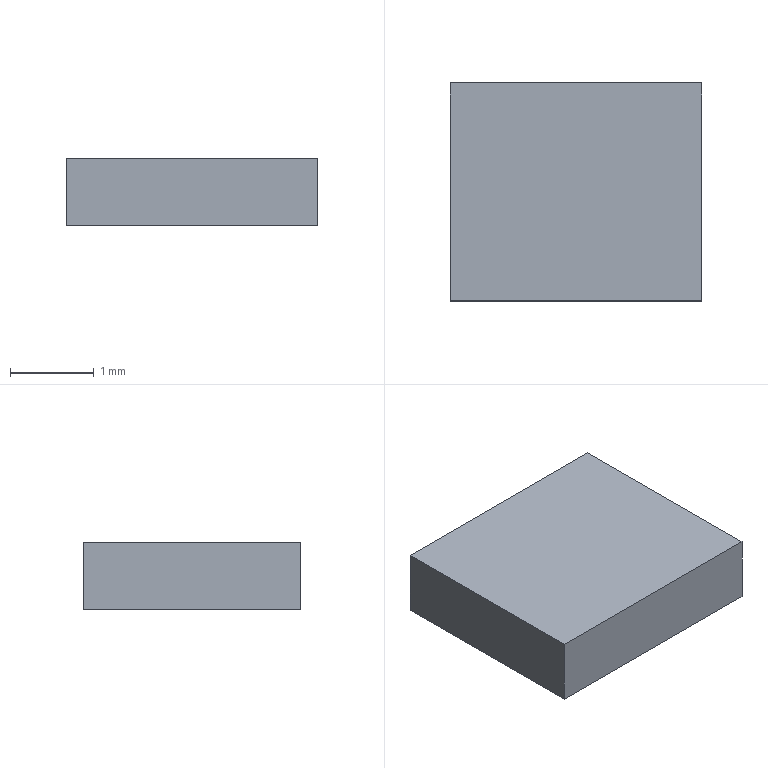Part | Creo | 1 solid | 6 faces | box 3 x 2.6 x 0.8 mm | volume 6.24 mm3 | plane 6
STEP:
#1=CARTESIAN_POINT('',(0.,0.,0.));
#2=DIRECTION('',(0.,0.,1.));
#3=DIRECTION('',(1.,0.,0.));
#4=AXIS2_PLACEMENT_3D('',#1,#2,#3);
#5=CARTESIAN_POINT('',(-1.5,1.3,0.));
#6=VERTEX_POINT('',#5);
#7=CARTESIAN_POINT('',(-1.5,-1.3,0.));
#8=VERTEX_POINT('',#7);
#9=CARTESIAN_POINT('',(-1.5,1.3,0.));
#10=DIRECTION('',(0.,-1.,0.));
#11=VECTOR('',#10,2.6);
#12=LINE('',#9,#11);
#13=EDGE_CURVE('',#6,#8,#12,.T.);
#14=ORIENTED_EDGE('',*,*,#13,.T.);
#15=CARTESIAN_POINT('',(1.5,-1.3,0.));
#16=VERTEX_POINT('',#15);
#17=CARTESIAN_POINT('',(-1.5,-1.3,0.));
#18=DIRECTION('',(1.,0.,0.));
#19=VECTOR('',#18,3.);
#20=LINE('',#17,#19);
#21=EDGE_CURVE('',#8,#16,#20,.T.);
#22=ORIENTED_EDGE('',*,*,#21,.T.);
#23=CARTESIAN_POINT('',(1.5,1.3,0.));
#24=VERTEX_POINT('',#23);
#25=CARTESIAN_POINT('',(1.5,-1.3,0.));
#26=DIRECTION('',(0.,1.,0.));
#27=VECTOR('',#26,2.6);
#28=LINE('',#25,#27);
#29=EDGE_CURVE('',#16,#24,#28,.T.);
#30=ORIENTED_EDGE('',*,*,#29,.T.);
#31=CARTESIAN_POINT('',(1.5,1.3,0.));
#32=DIRECTION('',(-1.,0.,0.));
#33=VECTOR('',#32,3.);
#34=LINE('',#31,#33);
#35=EDGE_CURVE('',#24,#6,#34,.T.);
#36=ORIENTED_EDGE('',*,*,#35,.T.);
#37=EDGE_LOOP('',(#14,#22,#30,#36));
#38=FACE_OUTER_BOUND('',#37,.F.);
#39=CARTESIAN_POINT('',(0.,0.,0.));
#40=DIRECTION('',(0.,0.,1.));
#41=DIRECTION('',(1.,0.,0.));
#42=AXIS2_PLACEMENT_3D('',#39,#40,#41);
#43=PLANE('',#42);
#44=ADVANCED_FACE('',(#38),#43,.F.);
#45=ORIENTED_EDGE('',*,*,#13,.F.);
#46=CARTESIAN_POINT('',(-1.5,1.3,0.8));
#47=VERTEX_POINT('',#46);
#48=CARTESIAN_POINT('',(-1.5,1.3,0.));
#49=DIRECTION('',(0.,0.,1.));
#50=VECTOR('',#49,0.8);
#51=LINE('',#48,#50);
#52=EDGE_CURVE('',#6,#47,#51,.T.);
#53=ORIENTED_EDGE('',*,*,#52,.T.);
#54=CARTESIAN_POINT('',(-1.5,-1.3,0.8));
#55=VERTEX_POINT('',#54);
#56=CARTESIAN_POINT('',(-1.5,1.3,0.8));
#57=DIRECTION('',(0.,-1.,0.));
#58=VECTOR('',#57,2.6);
#59=LINE('',#56,#58);
#60=EDGE_CURVE('',#47,#55,#59,.T.);
#61=ORIENTED_EDGE('',*,*,#60,.T.);
#62=CARTESIAN_POINT('',(-1.5,-1.3,0.));
#63=DIRECTION('',(0.,0.,1.));
#64=VECTOR('',#63,0.8);
#65=LINE('',#62,#64);
#66=EDGE_CURVE('',#8,#55,#65,.T.);
#67=ORIENTED_EDGE('',*,*,#66,.F.);
#68=EDGE_LOOP('',(#45,#53,#61,#67));
#69=FACE_OUTER_BOUND('',#68,.F.);
#70=CARTESIAN_POINT('',(-1.5,1.3,0.));
#71=DIRECTION('',(-1.,0.,0.));
#72=DIRECTION('',(0.,-1.,0.));
#73=AXIS2_PLACEMENT_3D('',#70,#71,#72);
#74=PLANE('',#73);
#75=ADVANCED_FACE('',(#69),#74,.T.);
#76=ORIENTED_EDGE('',*,*,#35,.F.);
#77=CARTESIAN_POINT('',(1.5,1.3,0.8));
#78=VERTEX_POINT('',#77);
#79=CARTESIAN_POINT('',(1.5,1.3,0.));
#80=DIRECTION('',(0.,0.,1.));
#81=VECTOR('',#80,0.8);
#82=LINE('',#79,#81);
#83=EDGE_CURVE('',#24,#78,#82,.T.);
#84=ORIENTED_EDGE('',*,*,#83,.T.);
#85=CARTESIAN_POINT('',(1.5,1.3,0.8));
#86=DIRECTION('',(-1.,0.,0.));
#87=VECTOR('',#86,3.);
#88=LINE('',#85,#87);
#89=EDGE_CURVE('',#78,#47,#88,.T.);
#90=ORIENTED_EDGE('',*,*,#89,.T.);
#91=ORIENTED_EDGE('',*,*,#52,.F.);
#92=EDGE_LOOP('',(#76,#84,#90,#91));
#93=FACE_OUTER_BOUND('',#92,.F.);
#94=CARTESIAN_POINT('',(1.5,1.3,0.));
#95=DIRECTION('',(0.,1.,0.));
#96=DIRECTION('',(-1.,0.,0.));
#97=AXIS2_PLACEMENT_3D('',#94,#95,#96);
#98=PLANE('',#97);
#99=ADVANCED_FACE('',(#93),#98,.T.);
#100=ORIENTED_EDGE('',*,*,#29,.F.);
#101=CARTESIAN_POINT('',(1.5,-1.3,0.8));
#102=VERTEX_POINT('',#101);
#103=CARTESIAN_POINT('',(1.5,-1.3,0.));
#104=DIRECTION('',(0.,0.,1.));
#105=VECTOR('',#104,0.8);
#106=LINE('',#103,#105);
#107=EDGE_CURVE('',#16,#102,#106,.T.);
#108=ORIENTED_EDGE('',*,*,#107,.T.);
#109=CARTESIAN_POINT('',(1.5,-1.3,0.8));
#110=DIRECTION('',(0.,1.,0.));
#111=VECTOR('',#110,2.6);
#112=LINE('',#109,#111);
#113=EDGE_CURVE('',#102,#78,#112,.T.);
#114=ORIENTED_EDGE('',*,*,#113,.T.);
#115=ORIENTED_EDGE('',*,*,#83,.F.);
#116=EDGE_LOOP('',(#100,#108,#114,#115));
#117=FACE_OUTER_BOUND('',#116,.F.);
#118=CARTESIAN_POINT('',(1.5,-1.3,0.));
#119=DIRECTION('',(1.,0.,0.));
#120=DIRECTION('',(0.,1.,0.));
#121=AXIS2_PLACEMENT_3D('',#118,#119,#120);
#122=PLANE('',#121);
#123=ADVANCED_FACE('',(#117),#122,.T.);
#124=ORIENTED_EDGE('',*,*,#21,.F.);
#125=ORIENTED_EDGE('',*,*,#66,.T.);
#126=CARTESIAN_POINT('',(-1.5,-1.3,0.8));
#127=DIRECTION('',(1.,0.,0.));
#128=VECTOR('',#127,3.);
#129=LINE('',#126,#128);
#130=EDGE_CURVE('',#55,#102,#129,.T.);
#131=ORIENTED_EDGE('',*,*,#130,.T.);
#132=ORIENTED_EDGE('',*,*,#107,.F.);
#133=EDGE_LOOP('',(#124,#125,#131,#132));
#134=FACE_OUTER_BOUND('',#133,.F.);
#135=CARTESIAN_POINT('',(-1.5,-1.3,0.));
#136=DIRECTION('',(0.,-1.,0.));
#137=DIRECTION('',(1.,0.,0.));
#138=AXIS2_PLACEMENT_3D('',#135,#136,#137);
#139=PLANE('',#138);
#140=ADVANCED_FACE('',(#134),#139,.T.);
#141=ORIENTED_EDGE('',*,*,#60,.F.);
#142=ORIENTED_EDGE('',*,*,#89,.F.);
#143=ORIENTED_EDGE('',*,*,#113,.F.);
#144=ORIENTED_EDGE('',*,*,#130,.F.);
#145=EDGE_LOOP('',(#141,#142,#143,#144));
#146=FACE_OUTER_BOUND('',#145,.F.);
#147=CARTESIAN_POINT('',(0.,0.,0.8));
#148=DIRECTION('',(0.,0.,1.));
#149=DIRECTION('',(1.,0.,0.));
#150=AXIS2_PLACEMENT_3D('',#147,#148,#149);
#151=PLANE('',#150);
#152=ADVANCED_FACE('',(#146),#151,.T.);
#153=CLOSED_SHELL('',(#44,#75,#99,#123,#140,#152));
#154=MANIFOLD_SOLID_BREP('',#153);
#155=(LENGTH_UNIT()NAMED_UNIT(*)SI_UNIT(.MILLI.,.METRE.));
#156=UNCERTAINTY_MEASURE_WITH_UNIT(LENGTH_MEASURE(0.000405),#155,'','');
#157=(NAMED_UNIT(*)PLANE_ANGLE_UNIT()SI_UNIT($,.RADIAN.));
#158=PLANE_ANGLE_MEASURE_WITH_UNIT(PLANE_ANGLE_MEASURE(0.01745),#157);
#159=(CONVERSION_BASED_UNIT('DEGREE',#158)NAMED_UNIT(*)PLANE_ANGLE_UNIT());
#160=(NAMED_UNIT(*)SI_UNIT($,.STERADIAN.)SOLID_ANGLE_UNIT());
#161=(GEOMETRIC_REPRESENTATION_CONTEXT(3)GLOBAL_UNCERTAINTY_ASSIGNED_CONTEXT((#156))GLOBAL_UNIT_ASSIGNED_CONTEXT((#155,#159,#160))REPRESENTATION_CONTEXT('',''));
#162=ADVANCED_BREP_SHAPE_REPRESENTATION('',(#4,#154),#161);